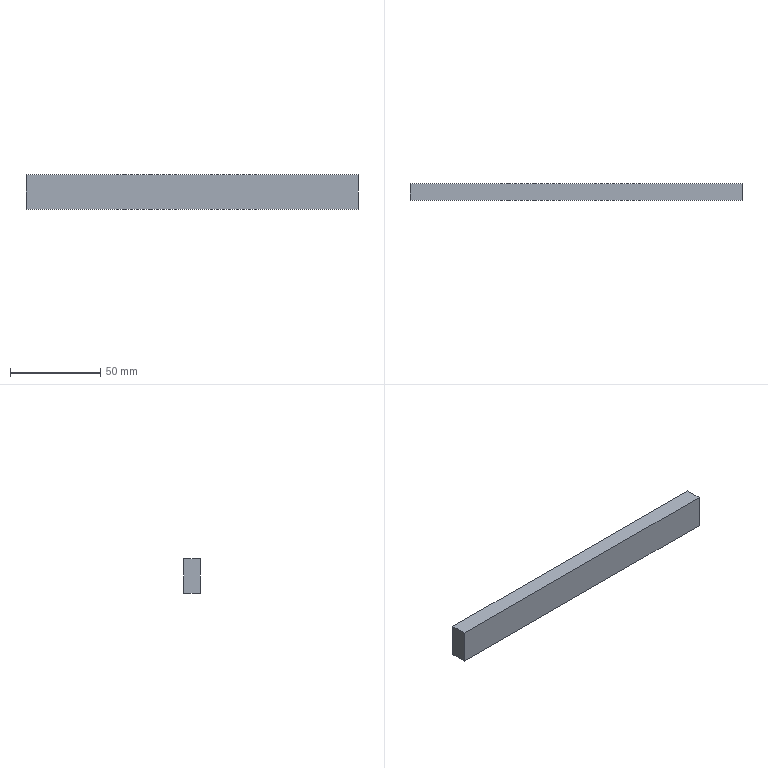Part | SolidWorks | features FlatPattern 1, SMBaseFlange 1, SheetMetal 1 | 1 solid | 6 faces | box 183.5 x 9 x 19 mm | volume 31378 mm3 | plane 6
STEP:
#1=CARTESIAN_POINT('',(91.75,0.,9.5));
#2=VERTEX_POINT('',#1);
#3=CARTESIAN_POINT('',(91.75,0.,-9.5));
#4=VERTEX_POINT('',#3);
#5=CARTESIAN_POINT('',(91.75,0.,-9.5));
#6=DIRECTION('',(0.,0.,-1.));
#7=VECTOR('',#6,1000.);
#8=LINE('',#5,#7);
#9=EDGE_CURVE('',#2,#4,#8,.T.);
#10=ORIENTED_EDGE('',*,*,#9,.T.);
#11=CARTESIAN_POINT('',(91.75,9.,-9.5));
#12=VERTEX_POINT('',#11);
#13=CARTESIAN_POINT('',(91.75,9.,-9.5));
#14=DIRECTION('',(0.,-1.,0.));
#15=VECTOR('',#14,1000.);
#16=LINE('',#13,#15);
#17=EDGE_CURVE('',#12,#4,#16,.T.);
#18=ORIENTED_EDGE('',*,*,#17,.F.);
#19=CARTESIAN_POINT('',(91.75,9.,9.5));
#20=VERTEX_POINT('',#19);
#21=CARTESIAN_POINT('',(91.75,9.,-9.5));
#22=DIRECTION('',(0.,0.,-1.));
#23=VECTOR('',#22,1000.);
#24=LINE('',#21,#23);
#25=EDGE_CURVE('',#20,#12,#24,.T.);
#26=ORIENTED_EDGE('',*,*,#25,.F.);
#27=CARTESIAN_POINT('',(91.75,9.,9.5));
#28=DIRECTION('',(0.,-1.,0.));
#29=VECTOR('',#28,1000.);
#30=LINE('',#27,#29);
#31=EDGE_CURVE('',#20,#2,#30,.T.);
#32=ORIENTED_EDGE('',*,*,#31,.T.);
#33=EDGE_LOOP('',(#10,#18,#26,#32));
#34=FACE_OUTER_BOUND('',#33,.T.);
#35=CARTESIAN_POINT('',(91.75,9.,-9.5));
#36=DIRECTION('',(-1.,0.,0.));
#37=DIRECTION('',(0.,0.,1.));
#38=AXIS2_PLACEMENT_3D('',#35,#36,#37);
#39=PLANE('',#38);
#40=ADVANCED_FACE('',(#34),#39,.F.);
#41=CARTESIAN_POINT('',(-91.75,0.,-9.5));
#42=VERTEX_POINT('',#41);
#43=CARTESIAN_POINT('',(-91.75,0.,-9.5));
#44=DIRECTION('',(-1.,0.,0.));
#45=VECTOR('',#44,1000.);
#46=LINE('',#43,#45);
#47=EDGE_CURVE('',#4,#42,#46,.T.);
#48=ORIENTED_EDGE('',*,*,#47,.T.);
#49=CARTESIAN_POINT('',(-91.75,9.,-9.5));
#50=VERTEX_POINT('',#49);
#51=CARTESIAN_POINT('',(-91.75,9.,-9.5));
#52=DIRECTION('',(0.,-1.,0.));
#53=VECTOR('',#52,1000.);
#54=LINE('',#51,#53);
#55=EDGE_CURVE('',#50,#42,#54,.T.);
#56=ORIENTED_EDGE('',*,*,#55,.F.);
#57=CARTESIAN_POINT('',(-91.75,9.,-9.5));
#58=DIRECTION('',(-1.,0.,0.));
#59=VECTOR('',#58,1000.);
#60=LINE('',#57,#59);
#61=EDGE_CURVE('',#12,#50,#60,.T.);
#62=ORIENTED_EDGE('',*,*,#61,.F.);
#63=ORIENTED_EDGE('',*,*,#17,.T.);
#64=EDGE_LOOP('',(#48,#56,#62,#63));
#65=FACE_OUTER_BOUND('',#64,.T.);
#66=CARTESIAN_POINT('',(-91.75,9.,-9.5));
#67=DIRECTION('',(0.,0.,1.));
#68=DIRECTION('',(1.,0.,0.));
#69=AXIS2_PLACEMENT_3D('',#66,#67,#68);
#70=PLANE('',#69);
#71=ADVANCED_FACE('',(#65),#70,.F.);
#72=CARTESIAN_POINT('',(-91.75,0.,9.5));
#73=VERTEX_POINT('',#72);
#74=CARTESIAN_POINT('',(-91.75,0.,-9.5));
#75=DIRECTION('',(0.,0.,1.));
#76=VECTOR('',#75,1000.);
#77=LINE('',#74,#76);
#78=EDGE_CURVE('',#42,#73,#77,.T.);
#79=ORIENTED_EDGE('',*,*,#78,.T.);
#80=CARTESIAN_POINT('',(-91.75,9.,9.5));
#81=VERTEX_POINT('',#80);
#82=CARTESIAN_POINT('',(-91.75,9.,9.5));
#83=DIRECTION('',(0.,-1.,0.));
#84=VECTOR('',#83,1000.);
#85=LINE('',#82,#84);
#86=EDGE_CURVE('',#81,#73,#85,.T.);
#87=ORIENTED_EDGE('',*,*,#86,.F.);
#88=CARTESIAN_POINT('',(-91.75,9.,-9.5));
#89=DIRECTION('',(0.,0.,1.));
#90=VECTOR('',#89,1000.);
#91=LINE('',#88,#90);
#92=EDGE_CURVE('',#50,#81,#91,.T.);
#93=ORIENTED_EDGE('',*,*,#92,.F.);
#94=ORIENTED_EDGE('',*,*,#55,.T.);
#95=EDGE_LOOP('',(#79,#87,#93,#94));
#96=FACE_OUTER_BOUND('',#95,.T.);
#97=CARTESIAN_POINT('',(-91.75,9.,-9.5));
#98=DIRECTION('',(1.,0.,0.));
#99=DIRECTION('',(0.,0.,-1.));
#100=AXIS2_PLACEMENT_3D('',#97,#98,#99);
#101=PLANE('',#100);
#102=ADVANCED_FACE('',(#96),#101,.F.);
#103=CARTESIAN_POINT('',(-91.75,0.,9.5));
#104=DIRECTION('',(1.,0.,0.));
#105=VECTOR('',#104,1000.);
#106=LINE('',#103,#105);
#107=EDGE_CURVE('',#73,#2,#106,.T.);
#108=ORIENTED_EDGE('',*,*,#107,.T.);
#109=ORIENTED_EDGE('',*,*,#31,.F.);
#110=CARTESIAN_POINT('',(-91.75,9.,9.5));
#111=DIRECTION('',(1.,0.,0.));
#112=VECTOR('',#111,1000.);
#113=LINE('',#110,#112);
#114=EDGE_CURVE('',#81,#20,#113,.T.);
#115=ORIENTED_EDGE('',*,*,#114,.F.);
#116=ORIENTED_EDGE('',*,*,#86,.T.);
#117=EDGE_LOOP('',(#108,#109,#115,#116));
#118=FACE_OUTER_BOUND('',#117,.T.);
#119=CARTESIAN_POINT('',(-91.75,9.,9.5));
#120=DIRECTION('',(0.,0.,-1.));
#121=DIRECTION('',(-1.,0.,0.));
#122=AXIS2_PLACEMENT_3D('',#119,#120,#121);
#123=PLANE('',#122);
#124=ADVANCED_FACE('',(#118),#123,.F.);
#125=ORIENTED_EDGE('',*,*,#25,.T.);
#126=ORIENTED_EDGE('',*,*,#61,.T.);
#127=ORIENTED_EDGE('',*,*,#92,.T.);
#128=ORIENTED_EDGE('',*,*,#114,.T.);
#129=EDGE_LOOP('',(#125,#126,#127,#128));
#130=FACE_OUTER_BOUND('',#129,.T.);
#131=CARTESIAN_POINT('',(0.,9.,0.));
#132=DIRECTION('',(0.,1.,0.));
#133=DIRECTION('',(0.,0.,1.));
#134=AXIS2_PLACEMENT_3D('',#131,#132,#133);
#135=PLANE('',#134);
#136=ADVANCED_FACE('',(#130),#135,.T.);
#137=ORIENTED_EDGE('',*,*,#9,.F.);
#138=ORIENTED_EDGE('',*,*,#107,.F.);
#139=ORIENTED_EDGE('',*,*,#78,.F.);
#140=ORIENTED_EDGE('',*,*,#47,.F.);
#141=EDGE_LOOP('',(#137,#138,#139,#140));
#142=FACE_OUTER_BOUND('',#141,.T.);
#143=CARTESIAN_POINT('',(0.,0.,0.));
#144=DIRECTION('',(0.,1.,0.));
#145=DIRECTION('',(0.,0.,1.));
#146=AXIS2_PLACEMENT_3D('',#143,#144,#145);
#147=PLANE('',#146);
#148=ADVANCED_FACE('',(#142),#147,.F.);
#149=CLOSED_SHELL('',(#40,#71,#102,#124,#136,#148));
#150=MANIFOLD_SOLID_BREP('',#149);
#151=CARTESIAN_POINT('',(0.,0.,0.));
#152=DIRECTION('',(0.,0.,1.));
#153=DIRECTION('',(1.,0.,0.));
#154=AXIS2_PLACEMENT_3D('',#151,#152,#153);
#155=(LENGTH_UNIT()NAMED_UNIT(*)SI_UNIT(.MILLI.,.METRE.));
#156=UNCERTAINTY_MEASURE_WITH_UNIT(LENGTH_MEASURE(0.00001),#155,'','');
#157=(NAMED_UNIT(*)PLANE_ANGLE_UNIT()SI_UNIT($,.RADIAN.));
#158=(NAMED_UNIT(*)SI_UNIT($,.STERADIAN.)SOLID_ANGLE_UNIT());
#159=(GEOMETRIC_REPRESENTATION_CONTEXT(3)GLOBAL_UNCERTAINTY_ASSIGNED_CONTEXT((#156))GLOBAL_UNIT_ASSIGNED_CONTEXT((#155,#157,#158))REPRESENTATION_CONTEXT('',''));
#160=ADVANCED_BREP_SHAPE_REPRESENTATION('',(#150,#154),#159);